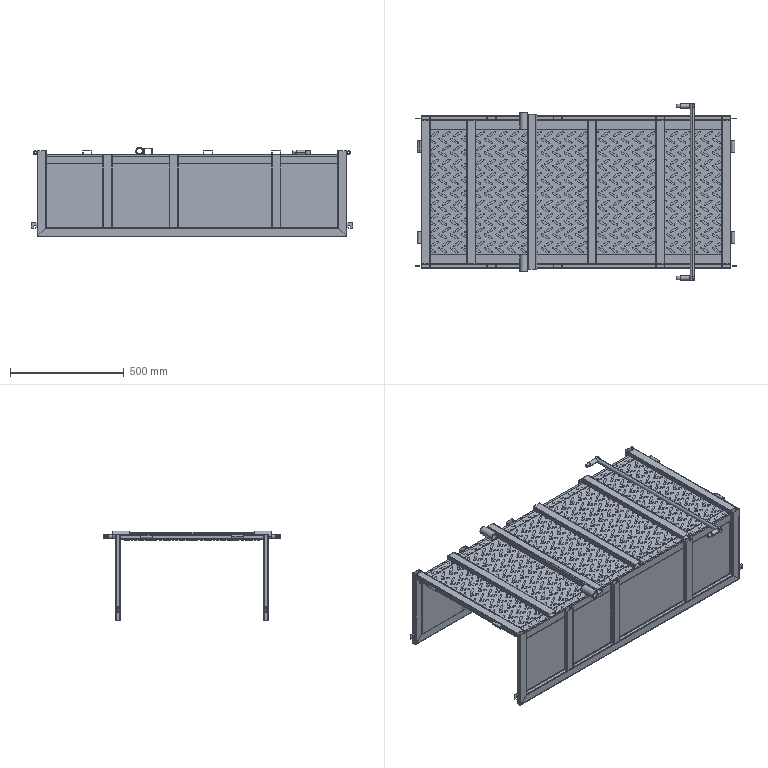Part | SolidWorks | 36 solids | 3622 faces | volume 6250840 mm3 | spline 2080 | plane 1316 | cylinder 202 | cone 24 | commonest cylinder face diameters 6 x72 2 x68 20 x16 11 x8 16 x8 4 x4